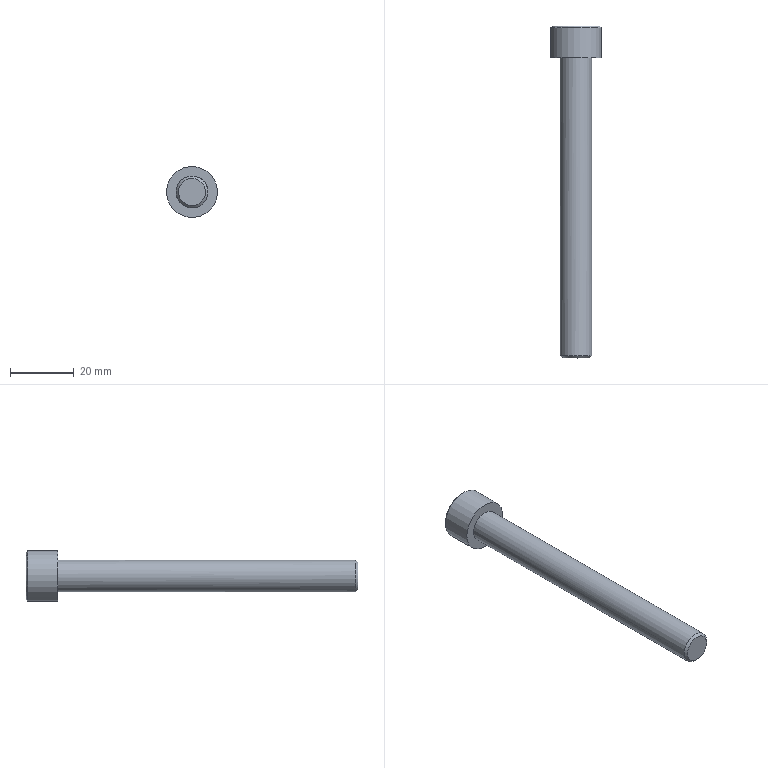Part | STEP file | solid 31 | 1 solid | 42 faces | box 16 x 104.2 x 16 mm | volume 9078 mm3 | plane 29 | other 8 | cone 3 | cylinder 2 | commonest cylinder face diameters 10 x1 16 x1